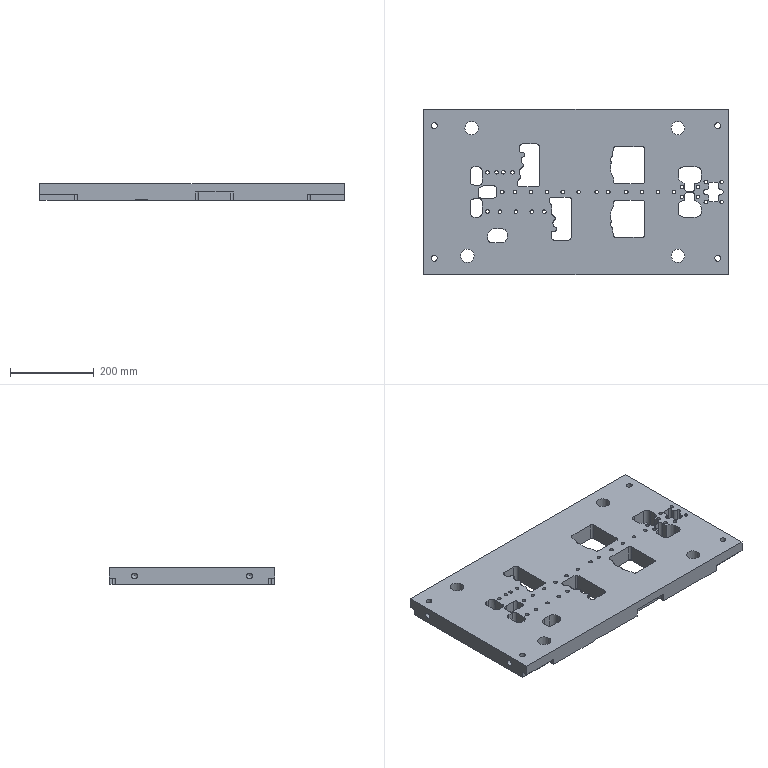Part | STEP file | PN_0025_id842_x_t | 1 solid | 622 faces | box 727.5 x 395 x 40 mm | volume 9281090 mm3 | plane 355 | cylinder 194 | cone 47 | spline 26 | commonest cylinder face diameters 10 x47 8.5 x40 6.8 x20 16 x20 8 x12 14 x12